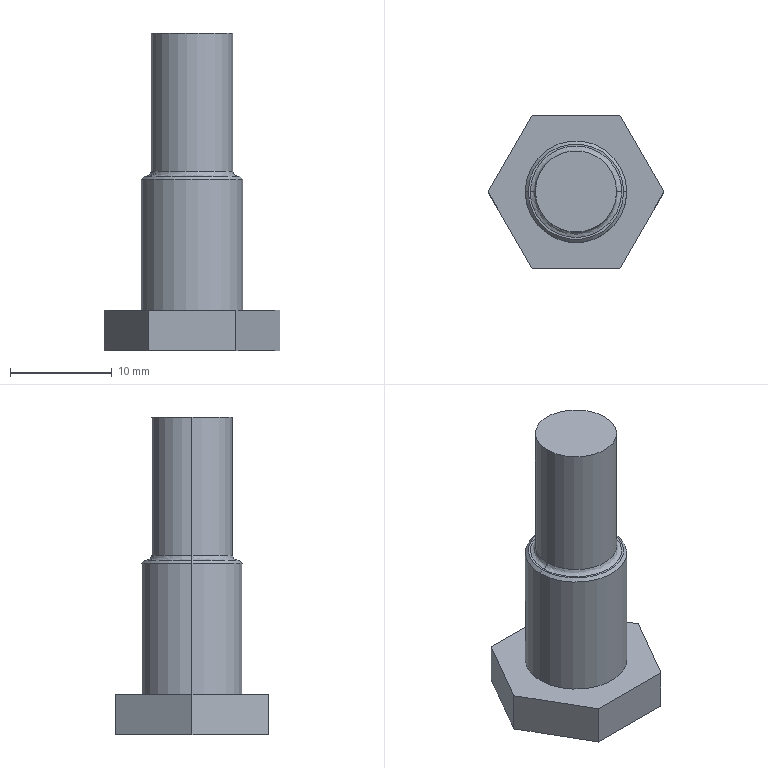Part | SolidWorks | features BaseBody 1 | 1 solid | 18 faces | box 17.321 x 15 x 31.3 mm | volume 2525 mm3 | plane 10 | cylinder 4 | spline 2 | cone 2 | commonest cylinder face diameters 8 x2 10 x2
STEP:
#1=CARTESIAN_POINT('',(-4.5,0.,17.2));
#2=VERTEX_POINT('',#1);
#3=CARTESIAN_POINT('',(4.5,0.,17.2));
#4=VERTEX_POINT('',#3);
#5=CARTESIAN_POINT('',(-4.5,0.,17.2));
#6=CARTESIAN_POINT('',(-4.5,0.286,17.2));
#7=CARTESIAN_POINT('',(-4.461,0.7076,17.2));
#8=CARTESIAN_POINT('',(-4.345,1.186,17.2));
#9=CARTESIAN_POINT('',(-4.27,1.422,17.2));
#10=CARTESIAN_POINT('',(-4.235,1.523,17.2));
#11=CARTESIAN_POINT('',(-4.21,1.59,17.2));
#12=CARTESIAN_POINT('',(-4.198,1.621,17.2));
#13=CARTESIAN_POINT('',(-4.128,1.798,17.2));
#14=CARTESIAN_POINT('',(-4.034,2.004,17.2));
#15=CARTESIAN_POINT('',(-3.925,2.203,17.2));
#16=CARTESIAN_POINT('',(-3.848,2.334,17.2));
#17=CARTESIAN_POINT('',(-3.809,2.398,17.2));
#18=CARTESIAN_POINT('',(-3.597,2.722,17.2));
#19=CARTESIAN_POINT('',(-3.401,2.963,17.2));
#20=CARTESIAN_POINT('',(-3.072,3.292,17.2));
#21=CARTESIAN_POINT('',(-2.9,3.447,17.2));
#22=CARTESIAN_POINT('',(-2.716,3.589,17.2));
#23=CARTESIAN_POINT('',(-2.591,3.68,17.2));
#24=CARTESIAN_POINT('',(-2.526,3.725,17.2));
#25=CARTESIAN_POINT('',(-2.335,3.85,17.2));
#26=CARTESIAN_POINT('',(-2.139,3.964,17.2));
#27=CARTESIAN_POINT('',(-1.901,4.08,17.2));
#28=CARTESIAN_POINT('',(-1.779,4.134,17.2));
#29=CARTESIAN_POINT('',(-1.727,4.155,17.2));
#30=CARTESIAN_POINT('',(-1.692,4.17,17.2));
#31=CARTESIAN_POINT('',(-1.673,4.177,17.2));
#32=CARTESIAN_POINT('',(-1.125,4.395,17.2));
#33=CARTESIAN_POINT('',(-0.5719,4.5,17.2));
#34=CARTESIAN_POINT('',(0.2859,4.5,17.2));
#35=CARTESIAN_POINT('',(0.7075,4.461,17.2));
#36=CARTESIAN_POINT('',(1.186,4.345,17.2));
#37=CARTESIAN_POINT('',(1.422,4.27,17.2));
#38=CARTESIAN_POINT('',(1.523,4.235,17.2));
#39=CARTESIAN_POINT('',(1.59,4.21,17.2));
#40=CARTESIAN_POINT('',(1.621,4.198,17.2));
#41=CARTESIAN_POINT('',(1.798,4.128,17.2));
#42=CARTESIAN_POINT('',(2.004,4.034,17.2));
#43=CARTESIAN_POINT('',(2.203,3.925,17.2));
#44=CARTESIAN_POINT('',(2.334,3.848,17.2));
#45=CARTESIAN_POINT('',(2.398,3.809,17.2));
#46=CARTESIAN_POINT('',(2.722,3.597,17.2));
#47=CARTESIAN_POINT('',(2.963,3.401,17.2));
#48=CARTESIAN_POINT('',(3.292,3.072,17.2));
#49=CARTESIAN_POINT('',(3.447,2.9,17.2));
#50=CARTESIAN_POINT('',(3.589,2.716,17.2));
#51=CARTESIAN_POINT('',(3.68,2.591,17.2));
#52=CARTESIAN_POINT('',(3.725,2.526,17.2));
#53=CARTESIAN_POINT('',(3.85,2.335,17.2));
#54=CARTESIAN_POINT('',(3.964,2.139,17.2));
#55=CARTESIAN_POINT('',(4.08,1.901,17.2));
#56=CARTESIAN_POINT('',(4.134,1.779,17.2));
#57=CARTESIAN_POINT('',(4.155,1.727,17.2));
#58=CARTESIAN_POINT('',(4.17,1.692,17.2));
#59=CARTESIAN_POINT('',(4.177,1.673,17.2));
#60=CARTESIAN_POINT('',(4.395,1.125,17.2));
#61=CARTESIAN_POINT('',(4.5,0.5724,17.2));
#62=CARTESIAN_POINT('',(4.5,0.,17.2));
#63=B_SPLINE_CURVE_WITH_KNOTS('',3,(#5,#6,#7,#8,#9,#10,#11,#12,#13,#14,#15,#16,#17,#18,#19,#20,#21,#22,#23,#24,#25,#26,#27,#28,#29,#30,#31,#32,#33,#34,#35,#36,#37,#38,#39,#40,#41,#42,#43,#44,#45,#46,#47,#48,#49,#50,#51,#52,#53,#54,#55,#56,#57,#58,#59,#60,#61,#62),.UNSPECIFIED.,.F.,.F.,(4,1,1,1,2,2,1,2,2,2,1,2,2,1,1,1,2,2,2,1,1,1,2,2,1,2,2,2,1,2,2,1,1,1,2,2,4),(0.,0.0625,0.09375,0.1094,0.1172,0.125,0.1562,0.1719,0.1875,0.25,0.2812,0.2969,0.3125,0.3437,0.3594,0.3672,0.3711,0.375,0.5,0.5625,0.5937,0.6094,0.6172,0.625,0.6562,0.6719,0.6875,0.75,0.7812,0.7969,0.8125,0.8437,0.8594,0.8672,0.8711,0.875,1.),.UNSPECIFIED.);
#64=EDGE_CURVE('',#2,#4,#63,.T.);
#65=ORIENTED_EDGE('',*,*,#64,.F.);
#66=CARTESIAN_POINT('',(-4.,0.,17.7));
#67=VERTEX_POINT('',#66);
#68=CARTESIAN_POINT('',(-4.5,0.,17.7));
#69=DIRECTION('',(0.,-1.,0.));
#70=DIRECTION('',(-1.,0.,0.));
#71=AXIS2_PLACEMENT_3D('',#68,#69,#70);
#72=CIRCLE('',#71,0.5);
#73=EDGE_CURVE('',#2,#67,#72,.T.);
#74=ORIENTED_EDGE('',*,*,#73,.T.);
#75=CARTESIAN_POINT('',(4.,0.,17.7));
#76=VERTEX_POINT('',#75);
#77=CARTESIAN_POINT('',(0.,0.,17.7));
#78=DIRECTION('',(0.,0.,1.));
#79=DIRECTION('',(1.,0.,0.));
#80=AXIS2_PLACEMENT_3D('',#77,#78,#79);
#81=CIRCLE('',#80,4.);
#82=EDGE_CURVE('',#76,#67,#81,.T.);
#83=ORIENTED_EDGE('',*,*,#82,.F.);
#84=CARTESIAN_POINT('',(4.5,0.,17.7));
#85=DIRECTION('',(0.,1.,0.));
#86=DIRECTION('',(1.,0.,0.));
#87=AXIS2_PLACEMENT_3D('',#84,#85,#86);
#88=CIRCLE('',#87,0.5);
#89=EDGE_CURVE('',#4,#76,#88,.T.);
#90=ORIENTED_EDGE('',*,*,#89,.F.);
#91=EDGE_LOOP('',(#65,#74,#83,#90));
#92=FACE_OUTER_BOUND('',#91,.T.);
#93=CARTESIAN_POINT('',(4.5,0.,17.2));
#94=CARTESIAN_POINT('',(4.5,9.,17.2));
#95=CARTESIAN_POINT('',(-4.5,9.,17.2));
#96=CARTESIAN_POINT('',(-4.5,0.,17.2));
#97=CARTESIAN_POINT('',(4.207,0.,17.2));
#98=CARTESIAN_POINT('',(4.207,8.414,17.2));
#99=CARTESIAN_POINT('',(-4.207,8.414,17.2));
#100=CARTESIAN_POINT('',(-4.207,0.,17.2));
#101=CARTESIAN_POINT('',(4.,0.,17.407));
#102=CARTESIAN_POINT('',(4.,8.,17.407));
#103=CARTESIAN_POINT('',(-4.,8.,17.407));
#104=CARTESIAN_POINT('',(-4.,0.,17.407));
#105=CARTESIAN_POINT('',(4.,0.,17.7));
#106=CARTESIAN_POINT('',(4.,8.,17.7));
#107=CARTESIAN_POINT('',(-4.,8.,17.7));
#108=CARTESIAN_POINT('',(-4.,0.,17.7));
#109=(BOUNDED_SURFACE()B_SPLINE_SURFACE(3,3,((#93,#94,#95,#96),(#97,#98,#99,#100),(#101,#102,#103,#104),(#105,#106,#107,#108)),.UNSPECIFIED.,.F.,.F.,.T.)B_SPLINE_SURFACE_WITH_KNOTS((4,4),(4,4),(0.,1.),(0.,1.),.UNSPECIFIED.)GEOMETRIC_REPRESENTATION_ITEM()RATIONAL_B_SPLINE_SURFACE(((1.,0.3333,0.3333,1.),(0.8047,0.2682,0.2682,0.8047),(0.8047,0.2682,0.2682,0.8047),(1.,0.3333,0.3333,1.)))REPRESENTATION_ITEM('')SURFACE());
#110=ADVANCED_FACE('',(#92),#109,.F.);
#111=CARTESIAN_POINT('',(-5.,0.,16.9));
#112=VERTEX_POINT('',#111);
#113=CARTESIAN_POINT('',(5.,0.,16.9));
#114=VERTEX_POINT('',#113);
#115=CARTESIAN_POINT('',(0.,0.,16.9));
#116=DIRECTION('',(0.,0.,-1.));
#117=DIRECTION('',(-1.,0.,0.));
#118=AXIS2_PLACEMENT_3D('',#115,#116,#117);
#119=CIRCLE('',#118,5.);
#120=EDGE_CURVE('',#112,#114,#119,.T.);
#121=ORIENTED_EDGE('',*,*,#120,.T.);
#122=CARTESIAN_POINT('',(5.,0.,4.));
#123=VERTEX_POINT('',#122);
#124=CARTESIAN_POINT('',(5.,0.,17.));
#125=DIRECTION('',(0.,0.,-1.));
#126=VECTOR('',#125,1000.);
#127=LINE('',#124,#126);
#128=EDGE_CURVE('',#114,#123,#127,.T.);
#129=ORIENTED_EDGE('',*,*,#128,.T.);
#130=CARTESIAN_POINT('',(-5.,0.,4.));
#131=VERTEX_POINT('',#130);
#132=CARTESIAN_POINT('',(0.,0.,4.));
#133=DIRECTION('',(0.,0.,1.));
#134=DIRECTION('',(-1.,0.,0.));
#135=AXIS2_PLACEMENT_3D('',#132,#133,#134);
#136=CIRCLE('',#135,5.);
#137=EDGE_CURVE('',#123,#131,#136,.T.);
#138=ORIENTED_EDGE('',*,*,#137,.T.);
#139=CARTESIAN_POINT('',(-5.,0.,17.));
#140=DIRECTION('',(0.,0.,-1.));
#141=VECTOR('',#140,1000.);
#142=LINE('',#139,#141);
#143=EDGE_CURVE('',#112,#131,#142,.T.);
#144=ORIENTED_EDGE('',*,*,#143,.F.);
#145=EDGE_LOOP('',(#121,#129,#138,#144));
#146=FACE_OUTER_BOUND('',#145,.T.);
#147=CARTESIAN_POINT('',(0.,0.,17.));
#148=DIRECTION('',(0.,0.,-1.));
#149=DIRECTION('',(-1.,0.,0.));
#150=AXIS2_PLACEMENT_3D('',#147,#148,#149);
#151=CYLINDRICAL_SURFACE('',#150,5.);
#152=ADVANCED_FACE('',(#146),#151,.T.);
#153=CARTESIAN_POINT('',(-4.7,0.,17.2));
#154=VERTEX_POINT('',#153);
#155=CARTESIAN_POINT('',(4.7,0.,17.2));
#156=VERTEX_POINT('',#155);
#157=CARTESIAN_POINT('',(0.,0.,17.2));
#158=DIRECTION('',(0.,0.,-1.));
#159=DIRECTION('',(-1.,0.,0.));
#160=AXIS2_PLACEMENT_3D('',#157,#158,#159);
#161=CIRCLE('',#160,4.7);
#162=EDGE_CURVE('',#154,#156,#161,.T.);
#163=ORIENTED_EDGE('',*,*,#162,.T.);
#164=CARTESIAN_POINT('',(5.,0.,16.9));
#165=DIRECTION('',(0.7071,0.,-0.7071));
#166=VECTOR('',#165,1000.);
#167=LINE('',#164,#166);
#168=EDGE_CURVE('',#156,#114,#167,.T.);
#169=ORIENTED_EDGE('',*,*,#168,.T.);
#170=ORIENTED_EDGE('',*,*,#120,.F.);
#171=CARTESIAN_POINT('',(-5.,0.,16.9));
#172=DIRECTION('',(-0.7071,0.,-0.7071));
#173=VECTOR('',#172,1000.);
#174=LINE('',#171,#173);
#175=EDGE_CURVE('',#154,#112,#174,.T.);
#176=ORIENTED_EDGE('',*,*,#175,.F.);
#177=EDGE_LOOP('',(#163,#169,#170,#176));
#178=FACE_OUTER_BOUND('',#177,.T.);
#179=CARTESIAN_POINT('',(0.,0.,16.9));
#180=DIRECTION('',(0.,0.,-1.));
#181=DIRECTION('',(-1.,0.,0.));
#182=AXIS2_PLACEMENT_3D('',#179,#180,#181);
#183=CONICAL_SURFACE('',#182,5.,0.7854);
#184=ADVANCED_FACE('',(#178),#183,.T.);
#185=CARTESIAN_POINT('',(-4.,0.,31.3));
#186=VERTEX_POINT('',#185);
#187=CARTESIAN_POINT('',(4.,0.,31.3));
#188=VERTEX_POINT('',#187);
#189=CARTESIAN_POINT('',(0.,0.,31.3));
#190=DIRECTION('',(0.,0.,-1.));
#191=DIRECTION('',(-1.,0.,0.));
#192=AXIS2_PLACEMENT_3D('',#189,#190,#191);
#193=CIRCLE('',#192,4.);
#194=EDGE_CURVE('',#186,#188,#193,.T.);
#195=ORIENTED_EDGE('',*,*,#194,.T.);
#196=CARTESIAN_POINT('',(4.,0.,31.3));
#197=DIRECTION('',(0.,0.,-1.));
#198=VECTOR('',#197,1000.);
#199=LINE('',#196,#198);
#200=EDGE_CURVE('',#188,#76,#199,.T.);
#201=ORIENTED_EDGE('',*,*,#200,.T.);
#202=ORIENTED_EDGE('',*,*,#82,.T.);
#203=CARTESIAN_POINT('',(-4.,0.,31.3));
#204=DIRECTION('',(0.,0.,-1.));
#205=VECTOR('',#204,1000.);
#206=LINE('',#203,#205);
#207=EDGE_CURVE('',#186,#67,#206,.T.);
#208=ORIENTED_EDGE('',*,*,#207,.F.);
#209=EDGE_LOOP('',(#195,#201,#202,#208));
#210=FACE_OUTER_BOUND('',#209,.T.);
#211=CARTESIAN_POINT('',(0.,0.,31.3));
#212=DIRECTION('',(0.,0.,-1.));
#213=DIRECTION('',(-1.,0.,0.));
#214=AXIS2_PLACEMENT_3D('',#211,#212,#213);
#215=CYLINDRICAL_SURFACE('',#214,4.);
#216=ADVANCED_FACE('',(#210),#215,.T.);
#217=ORIENTED_EDGE('',*,*,#128,.F.);
#218=CARTESIAN_POINT('',(0.,0.,16.9));
#219=DIRECTION('',(0.,0.,-1.));
#220=DIRECTION('',(-1.,0.,0.));
#221=AXIS2_PLACEMENT_3D('',#218,#219,#220);
#222=CIRCLE('',#221,5.);
#223=EDGE_CURVE('',#114,#112,#222,.T.);
#224=ORIENTED_EDGE('',*,*,#223,.T.);
#225=ORIENTED_EDGE('',*,*,#143,.T.);
#226=CARTESIAN_POINT('',(0.,0.,4.));
#227=DIRECTION('',(0.,0.,1.));
#228=DIRECTION('',(-1.,0.,0.));
#229=AXIS2_PLACEMENT_3D('',#226,#227,#228);
#230=CIRCLE('',#229,5.);
#231=EDGE_CURVE('',#131,#123,#230,.T.);
#232=ORIENTED_EDGE('',*,*,#231,.T.);
#233=EDGE_LOOP('',(#217,#224,#225,#232));
#234=FACE_OUTER_BOUND('',#233,.T.);
#235=CARTESIAN_POINT('',(0.,0.,17.));
#236=DIRECTION('',(0.,0.,-1.));
#237=DIRECTION('',(-1.,0.,0.));
#238=AXIS2_PLACEMENT_3D('',#235,#236,#237);
#239=CYLINDRICAL_SURFACE('',#238,5.);
#240=ADVANCED_FACE('',(#234),#239,.T.);
#241=CARTESIAN_POINT('',(-4.33,-7.5,4.));
#242=VERTEX_POINT('',#241);
#243=CARTESIAN_POINT('',(4.33,-7.5,4.));
#244=VERTEX_POINT('',#243);
#245=CARTESIAN_POINT('',(0.,-7.5,4.));
#246=DIRECTION('',(1.,0.,0.));
#247=VECTOR('',#246,1000.);
#248=LINE('',#245,#247);
#249=EDGE_CURVE('',#242,#244,#248,.T.);
#250=ORIENTED_EDGE('',*,*,#249,.T.);
#251=CARTESIAN_POINT('',(8.66,0.,4.));
#252=VERTEX_POINT('',#251);
#253=CARTESIAN_POINT('',(4.33,-7.5,4.));
#254=DIRECTION('',(0.5,0.866,0.));
#255=VECTOR('',#254,1000.);
#256=LINE('',#253,#255);
#257=EDGE_CURVE('',#244,#252,#256,.T.);
#258=ORIENTED_EDGE('',*,*,#257,.T.);
#259=CARTESIAN_POINT('',(4.33,7.5,4.));
#260=VERTEX_POINT('',#259);
#261=CARTESIAN_POINT('',(8.66,0.,4.));
#262=DIRECTION('',(-0.5,0.866,0.));
#263=VECTOR('',#262,1000.);
#264=LINE('',#261,#263);
#265=EDGE_CURVE('',#252,#260,#264,.T.);
#266=ORIENTED_EDGE('',*,*,#265,.T.);
#267=CARTESIAN_POINT('',(-4.33,7.5,4.));
#268=VERTEX_POINT('',#267);
#269=CARTESIAN_POINT('',(0.,7.5,4.));
#270=DIRECTION('',(-1.,0.,0.));
#271=VECTOR('',#270,1000.);
#272=LINE('',#269,#271);
#273=EDGE_CURVE('',#260,#268,#272,.T.);
#274=ORIENTED_EDGE('',*,*,#273,.T.);
#275=CARTESIAN_POINT('',(-8.66,0.,4.));
#276=VERTEX_POINT('',#275);
#277=CARTESIAN_POINT('',(-4.33,7.5,4.));
#278=DIRECTION('',(-0.5,-0.866,0.));
#279=VECTOR('',#278,1000.);
#280=LINE('',#277,#279);
#281=EDGE_CURVE('',#268,#276,#280,.T.);
#282=ORIENTED_EDGE('',*,*,#281,.T.);
#283=CARTESIAN_POINT('',(-8.66,0.,4.));
#284=DIRECTION('',(0.5,-0.866,0.));
#285=VECTOR('',#284,1000.);
#286=LINE('',#283,#285);
#287=EDGE_CURVE('',#276,#242,#286,.T.);
#288=ORIENTED_EDGE('',*,*,#287,.T.);
#289=EDGE_LOOP('',(#250,#258,#266,#274,#282,#288));
#290=FACE_OUTER_BOUND('',#289,.T.);
#291=ORIENTED_EDGE('',*,*,#231,.F.);
#292=ORIENTED_EDGE('',*,*,#137,.F.);
#293=EDGE_LOOP('',(#291,#292));
#294=FACE_BOUND('',#293,.T.);
#295=CARTESIAN_POINT('',(0.,0.,4.));
#296=DIRECTION('',(0.,0.,1.));
#297=DIRECTION('',(1.,0.,0.));
#298=AXIS2_PLACEMENT_3D('',#295,#296,#297);
#299=PLANE('',#298);
#300=ADVANCED_FACE('',(#290,#294),#299,.T.);
#301=ORIENTED_EDGE('',*,*,#168,.F.);
#302=CARTESIAN_POINT('',(0.,0.,17.2));
#303=DIRECTION('',(0.,0.,-1.));
#304=DIRECTION('',(-1.,0.,0.));
#305=AXIS2_PLACEMENT_3D('',#302,#303,#304);
#306=CIRCLE('',#305,4.7);
#307=EDGE_CURVE('',#156,#154,#306,.T.);
#308=ORIENTED_EDGE('',*,*,#307,.T.);
#309=ORIENTED_EDGE('',*,*,#175,.T.);
#310=ORIENTED_EDGE('',*,*,#223,.F.);
#311=EDGE_LOOP('',(#301,#308,#309,#310));
#312=FACE_OUTER_BOUND('',#311,.T.);
#313=CARTESIAN_POINT('',(0.,0.,16.9));
#314=DIRECTION('',(0.,0.,-1.));
#315=DIRECTION('',(-1.,0.,0.));
#316=AXIS2_PLACEMENT_3D('',#313,#314,#315);
#317=CONICAL_SURFACE('',#316,5.,0.7854);
#318=ADVANCED_FACE('',(#312),#317,.T.);
#319=CARTESIAN_POINT('',(8.66,0.,0.));
#320=VERTEX_POINT('',#319);
#321=CARTESIAN_POINT('',(8.66,0.,4.));
#322=DIRECTION('',(0.,0.,-1.));
#323=VECTOR('',#322,1000.);
#324=LINE('',#321,#323);
#325=EDGE_CURVE('',#252,#320,#324,.T.);
#326=ORIENTED_EDGE('',*,*,#325,.F.);
#327=ORIENTED_EDGE('',*,*,#257,.F.);
#328=CARTESIAN_POINT('',(4.33,-7.5,0.));
#329=VERTEX_POINT('',#328);
#330=CARTESIAN_POINT('',(4.33,-7.5,4.));
#331=DIRECTION('',(0.,0.,1.));
#332=VECTOR('',#331,1000.);
#333=LINE('',#330,#332);
#334=EDGE_CURVE('',#329,#244,#333,.T.);
#335=ORIENTED_EDGE('',*,*,#334,.F.);
#336=CARTESIAN_POINT('',(4.33,-7.5,0.));
#337=DIRECTION('',(-0.5,-0.866,0.));
#338=VECTOR('',#337,1000.);
#339=LINE('',#336,#338);
#340=EDGE_CURVE('',#320,#329,#339,.T.);
#341=ORIENTED_EDGE('',*,*,#340,.F.);
#342=EDGE_LOOP('',(#326,#327,#335,#341));
#343=FACE_OUTER_BOUND('',#342,.T.);
#344=CARTESIAN_POINT('',(4.33,-7.5,4.));
#345=DIRECTION('',(-0.866,0.5,0.));
#346=DIRECTION('',(-0.5,-0.866,0.));
#347=AXIS2_PLACEMENT_3D('',#344,#345,#346);
#348=PLANE('',#347);
#349=ADVANCED_FACE('',(#343),#348,.F.);
#350=ORIENTED_EDGE('',*,*,#334,.T.);
#351=ORIENTED_EDGE('',*,*,#249,.F.);
#352=CARTESIAN_POINT('',(-4.33,-7.5,0.));
#353=VERTEX_POINT('',#352);
#354=CARTESIAN_POINT('',(-4.33,-7.5,4.));
#355=DIRECTION('',(0.,0.,1.));
#356=VECTOR('',#355,1000.);
#357=LINE('',#354,#356);
#358=EDGE_CURVE('',#353,#242,#357,.T.);
#359=ORIENTED_EDGE('',*,*,#358,.F.);
#360=CARTESIAN_POINT('',(-4.33,-7.5,0.));
#361=DIRECTION('',(-1.,0.,0.));
#362=VECTOR('',#361,1000.);
#363=LINE('',#360,#362);
#364=EDGE_CURVE('',#329,#353,#363,.T.);
#365=ORIENTED_EDGE('',*,*,#364,.F.);
#366=EDGE_LOOP('',(#350,#351,#359,#365));
#367=FACE_OUTER_BOUND('',#366,.T.);
#368=CARTESIAN_POINT('',(-4.33,-7.5,4.));
#369=DIRECTION('',(0.,1.,0.));
#370=DIRECTION('',(-1.,0.,0.));
#371=AXIS2_PLACEMENT_3D('',#368,#369,#370);
#372=PLANE('',#371);
#373=ADVANCED_FACE('',(#367),#372,.F.);
#374=ORIENTED_EDGE('',*,*,#358,.T.);
#375=ORIENTED_EDGE('',*,*,#287,.F.);
#376=CARTESIAN_POINT('',(-8.66,0.,0.));
#377=VERTEX_POINT('',#376);
#378=CARTESIAN_POINT('',(-8.66,0.,4.));
#379=DIRECTION('',(0.,0.,1.));
#380=VECTOR('',#379,1000.);
#381=LINE('',#378,#380);
#382=EDGE_CURVE('',#377,#276,#381,.T.);
#383=ORIENTED_EDGE('',*,*,#382,.F.);
#384=CARTESIAN_POINT('',(-8.66,0.,0.));
#385=DIRECTION('',(-0.5,0.866,0.));
#386=VECTOR('',#385,1000.);
#387=LINE('',#384,#386);
#388=EDGE_CURVE('',#353,#377,#387,.T.);
#389=ORIENTED_EDGE('',*,*,#388,.F.);
#390=EDGE_LOOP('',(#374,#375,#383,#389));
#391=FACE_OUTER_BOUND('',#390,.T.);
#392=CARTESIAN_POINT('',(-8.66,0.,4.));
#393=DIRECTION('',(0.866,0.5,0.));
#394=DIRECTION('',(-0.5,0.866,0.));
#395=AXIS2_PLACEMENT_3D('',#392,#393,#394);
#396=PLANE('',#395);
#397=ADVANCED_FACE('',(#391),#396,.F.);
#398=ORIENTED_EDGE('',*,*,#382,.T.);
#399=ORIENTED_EDGE('',*,*,#281,.F.);
#400=CARTESIAN_POINT('',(-4.33,7.5,0.));
#401=VERTEX_POINT('',#400);
#402=CARTESIAN_POINT('',(-4.33,7.5,4.));
#403=DIRECTION('',(0.,0.,1.));
#404=VECTOR('',#403,1000.);
#405=LINE('',#402,#404);
#406=EDGE_CURVE('',#401,#268,#405,.T.);
#407=ORIENTED_EDGE('',*,*,#406,.F.);
#408=CARTESIAN_POINT('',(-4.33,7.5,0.));
#409=DIRECTION('',(0.5,0.866,0.));
#410=VECTOR('',#409,1000.);
#411=LINE('',#408,#410);
#412=EDGE_CURVE('',#377,#401,#411,.T.);
#413=ORIENTED_EDGE('',*,*,#412,.F.);
#414=EDGE_LOOP('',(#398,#399,#407,#413));
#415=FACE_OUTER_BOUND('',#414,.T.);
#416=CARTESIAN_POINT('',(-4.33,7.5,4.));
#417=DIRECTION('',(0.866,-0.5,0.));
#418=DIRECTION('',(0.5,0.866,0.));
#419=AXIS2_PLACEMENT_3D('',#416,#417,#418);
#420=PLANE('',#419);
#421=ADVANCED_FACE('',(#415),#420,.F.);
#422=ORIENTED_EDGE('',*,*,#406,.T.);
#423=ORIENTED_EDGE('',*,*,#273,.F.);
#424=CARTESIAN_POINT('',(4.33,7.5,0.));
#425=VERTEX_POINT('',#424);
#426=CARTESIAN_POINT('',(4.33,7.5,4.));
#427=DIRECTION('',(0.,0.,1.));
#428=VECTOR('',#427,1000.);
#429=LINE('',#426,#428);
#430=EDGE_CURVE('',#425,#260,#429,.T.);
#431=ORIENTED_EDGE('',*,*,#430,.F.);
#432=CARTESIAN_POINT('',(4.33,7.5,0.));
#433=DIRECTION('',(1.,0.,0.));
#434=VECTOR('',#433,1000.);
#435=LINE('',#432,#434);
#436=EDGE_CURVE('',#401,#425,#435,.T.);
#437=ORIENTED_EDGE('',*,*,#436,.F.);
#438=EDGE_LOOP('',(#422,#423,#431,#437));
#439=FACE_OUTER_BOUND('',#438,.T.);
#440=CARTESIAN_POINT('',(4.33,7.5,4.));
#441=DIRECTION('',(0.,-1.,0.));
#442=DIRECTION('',(0.,0.,-1.));
#443=AXIS2_PLACEMENT_3D('',#440,#441,#442);
#444=PLANE('',#443);
#445=ADVANCED_FACE('',(#439),#444,.F.);
#446=ORIENTED_EDGE('',*,*,#430,.T.);
#447=ORIENTED_EDGE('',*,*,#265,.F.);
#448=ORIENTED_EDGE('',*,*,#325,.T.);
#449=CARTESIAN_POINT('',(8.66,0.,0.));
#450=DIRECTION('',(0.5,-0.866,0.));
#451=VECTOR('',#450,1000.);
#452=LINE('',#449,#451);
#453=EDGE_CURVE('',#425,#320,#452,.T.);
#454=ORIENTED_EDGE('',*,*,#453,.F.);
#455=EDGE_LOOP('',(#446,#447,#448,#454));
#456=FACE_OUTER_BOUND('',#455,.T.);
#457=CARTESIAN_POINT('',(8.66,0.,4.));
#458=DIRECTION('',(-0.866,-0.5,0.));
#459=DIRECTION('',(0.5,-0.866,0.));
#460=AXIS2_PLACEMENT_3D('',#457,#458,#459);
#461=PLANE('',#460);
#462=ADVANCED_FACE('',(#456),#461,.F.);
#463=CARTESIAN_POINT('',(4.5,0.,17.2));
#464=CARTESIAN_POINT('',(4.5,-0.286,17.2));
#465=CARTESIAN_POINT('',(4.461,-0.7076,17.2));
#466=CARTESIAN_POINT('',(4.345,-1.186,17.2));
#467=CARTESIAN_POINT('',(4.27,-1.422,17.2));
#468=CARTESIAN_POINT('',(4.235,-1.523,17.2));
#469=CARTESIAN_POINT('',(4.21,-1.59,17.2));
#470=CARTESIAN_POINT('',(4.198,-1.621,17.2));
#471=CARTESIAN_POINT('',(4.128,-1.798,17.2));
#472=CARTESIAN_POINT('',(4.034,-2.004,17.2));
#473=CARTESIAN_POINT('',(3.925,-2.203,17.2));
#474=CARTESIAN_POINT('',(3.848,-2.334,17.2));
#475=CARTESIAN_POINT('',(3.809,-2.398,17.2));
#476=CARTESIAN_POINT('',(3.597,-2.722,17.2));
#477=CARTESIAN_POINT('',(3.401,-2.963,17.2));
#478=CARTESIAN_POINT('',(3.072,-3.292,17.2));
#479=CARTESIAN_POINT('',(2.9,-3.447,17.2));
#480=CARTESIAN_POINT('',(2.716,-3.589,17.2));
#481=CARTESIAN_POINT('',(2.591,-3.68,17.2));
#482=CARTESIAN_POINT('',(2.526,-3.725,17.2));
#483=CARTESIAN_POINT('',(2.335,-3.85,17.2));
#484=CARTESIAN_POINT('',(2.139,-3.964,17.2));
#485=CARTESIAN_POINT('',(1.901,-4.08,17.2));
#486=CARTESIAN_POINT('',(1.779,-4.134,17.2));
#487=CARTESIAN_POINT('',(1.727,-4.155,17.2));
#488=CARTESIAN_POINT('',(1.692,-4.17,17.2));
#489=CARTESIAN_POINT('',(1.673,-4.177,17.2));
#490=CARTESIAN_POINT('',(1.125,-4.395,17.2));
#491=CARTESIAN_POINT('',(0.5719,-4.5,17.2));
#492=CARTESIAN_POINT('',(-0.2859,-4.5,17.2));
#493=CARTESIAN_POINT('',(-0.7075,-4.461,17.2));
#494=CARTESIAN_POINT('',(-1.186,-4.345,17.2));
#495=CARTESIAN_POINT('',(-1.422,-4.27,17.2));
#496=CARTESIAN_POINT('',(-1.523,-4.235,17.2));
#497=CARTESIAN_POINT('',(-1.59,-4.21,17.2));
#498=CARTESIAN_POINT('',(-1.621,-4.198,17.2));
#499=CARTESIAN_POINT('',(-1.798,-4.128,17.2));
#500=CARTESIAN_POINT('',(-2.004,-4.034,17.2));
#501=CARTESIAN_POINT('',(-2.203,-3.925,17.2));
#502=CARTESIAN_POINT('',(-2.334,-3.848,17.2));
#503=CARTESIAN_POINT('',(-2.398,-3.809,17.2));
#504=CARTESIAN_POINT('',(-2.722,-3.597,17.2));
#505=CARTESIAN_POINT('',(-2.963,-3.401,17.2));
#506=CARTESIAN_POINT('',(-3.292,-3.072,17.2));
#507=CARTESIAN_POINT('',(-3.447,-2.9,17.2));
#508=CARTESIAN_POINT('',(-3.589,-2.716,17.2));
#509=CARTESIAN_POINT('',(-3.68,-2.591,17.2));
#510=CARTESIAN_POINT('',(-3.725,-2.526,17.2));
#511=CARTESIAN_POINT('',(-3.85,-2.335,17.2));
#512=CARTESIAN_POINT('',(-3.964,-2.139,17.2));
#513=CARTESIAN_POINT('',(-4.08,-1.901,17.2));
#514=CARTESIAN_POINT('',(-4.134,-1.779,17.2));
#515=CARTESIAN_POINT('',(-4.155,-1.727,17.2));
#516=CARTESIAN_POINT('',(-4.17,-1.692,17.2));
#517=CARTESIAN_POINT('',(-4.177,-1.673,17.2));
#518=CARTESIAN_POINT('',(-4.395,-1.125,17.2));
#519=CARTESIAN_POINT('',(-4.5,-0.5724,17.2));
#520=CARTESIAN_POINT('',(-4.5,0.,17.2));
#521=B_SPLINE_CURVE_WITH_KNOTS('',3,(#463,#464,#465,#466,#467,#468,#469,#470,#471,#472,#473,#474,#475,#476,#477,#478,#479,#480,#481,#482,#483,#484,#485,#486,#487,#488,#489,#490,#491,#492,#493,#494,#495,#496,#497,#498,#499,#500,#501,#502,#503,#504,#505,#506,#507,#508,#509,#510,#511,#512,#513,#514,#515,#516,#517,#518,#519,#520),.UNSPECIFIED.,.F.,.F.,(4,1,1,1,2,2,1,2,2,2,1,2,2,1,1,1,2,2,2,1,1,1,2,2,1,2,2,2,1,2,2,1,1,1,2,2,4),(0.,0.0625,0.09375,0.1094,0.1172,0.125,0.1562,0.1719,0.1875,0.25,0.2812,0.2969,0.3125,0.3437,0.3594,0.3672,0.3711,0.375,0.5,0.5625,0.5937,0.6094,0.6172,0.625,0.6562,0.6719,0.6875,0.75,0.7813,0.7969,0.8125,0.8438,0.8594,0.8672,0.8711,0.875,1.),.UNSPECIFIED.);
#522=EDGE_CURVE('',#4,#2,#521,.T.);
#523=ORIENTED_EDGE('',*,*,#522,.T.);
#524=ORIENTED_EDGE('',*,*,#64,.T.);
#525=EDGE_LOOP('',(#523,#524));
#526=FACE_BOUND('',#525,.T.);
#527=ORIENTED_EDGE('',*,*,#162,.F.);
#528=ORIENTED_EDGE('',*,*,#307,.F.);
#529=EDGE_LOOP('',(#527,#528));
#530=FACE_OUTER_BOUND('',#529,.T.);
#531=CARTESIAN_POINT('',(0.,0.,17.2));
#532=DIRECTION('',(0.,0.,1.));
#533=DIRECTION('',(1.,0.,0.));
#534=AXIS2_PLACEMENT_3D('',#531,#532,#533);
#535=PLANE('',#534);
#536=ADVANCED_FACE('',(#526,#530),#535,.T.);
#537=ORIENTED_EDGE('',*,*,#340,.T.);
#538=ORIENTED_EDGE('',*,*,#364,.T.);
#539=ORIENTED_EDGE('',*,*,#388,.T.);
#540=ORIENTED_EDGE('',*,*,#412,.T.);
#541=ORIENTED_EDGE('',*,*,#436,.T.);
#542=ORIENTED_EDGE('',*,*,#453,.T.);
#543=EDGE_LOOP('',(#537,#538,#539,#540,#541,#542));
#544=FACE_OUTER_BOUND('',#543,.T.);
#545=CARTESIAN_POINT('',(0.,0.,0.));
#546=DIRECTION('',(0.,0.,1.));
#547=DIRECTION('',(1.,0.,0.));
#548=AXIS2_PLACEMENT_3D('',#545,#546,#547);
#549=PLANE('',#548);
#550=ADVANCED_FACE('',(#544),#549,.F.);
#551=ORIENTED_EDGE('',*,*,#73,.F.);
#552=ORIENTED_EDGE('',*,*,#522,.F.);
#553=ORIENTED_EDGE('',*,*,#89,.T.);
#554=CARTESIAN_POINT('',(0.,0.,17.7));
#555=DIRECTION('',(0.,0.,1.));
#556=DIRECTION('',(1.,0.,0.));
#557=AXIS2_PLACEMENT_3D('',#554,#555,#556);
#558=CIRCLE('',#557,4.);
#559=EDGE_CURVE('',#67,#76,#558,.T.);
#560=ORIENTED_EDGE('',*,*,#559,.F.);
#561=EDGE_LOOP('',(#551,#552,#553,#560));
#562=FACE_OUTER_BOUND('',#561,.T.);
#563=CARTESIAN_POINT('',(-4.5,0.,17.2));
#564=CARTESIAN_POINT('',(-4.5,-9.,17.2));
#565=CARTESIAN_POINT('',(4.5,-9.,17.2));
#566=CARTESIAN_POINT('',(4.5,0.,17.2));
#567=CARTESIAN_POINT('',(-4.207,0.,17.2));
#568=CARTESIAN_POINT('',(-4.207,-8.414,17.2));
#569=CARTESIAN_POINT('',(4.207,-8.414,17.2));
#570=CARTESIAN_POINT('',(4.207,0.,17.2));
#571=CARTESIAN_POINT('',(-4.,0.,17.407));
#572=CARTESIAN_POINT('',(-4.,-8.,17.407));
#573=CARTESIAN_POINT('',(4.,-8.,17.407));
#574=CARTESIAN_POINT('',(4.,0.,17.407));
#575=CARTESIAN_POINT('',(-4.,0.,17.7));
#576=CARTESIAN_POINT('',(-4.,-8.,17.7));
#577=CARTESIAN_POINT('',(4.,-8.,17.7));
#578=CARTESIAN_POINT('',(4.,0.,17.7));
#579=(BOUNDED_SURFACE()B_SPLINE_SURFACE(3,3,((#563,#564,#565,#566),(#567,#568,#569,#570),(#571,#572,#573,#574),(#575,#576,#577,#578)),.UNSPECIFIED.,.F.,.F.,.F.)B_SPLINE_SURFACE_WITH_KNOTS((4,4),(4,4),(0.,1.),(0.,1.),.UNSPECIFIED.)GEOMETRIC_REPRESENTATION_ITEM()RATIONAL_B_SPLINE_SURFACE(((1.,0.3333,0.3333,1.),(0.8047,0.2682,0.2682,0.8047),(0.8047,0.2682,0.2682,0.8047),(1.,0.3333,0.3333,1.)))REPRESENTATION_ITEM('')SURFACE());
#580=ADVANCED_FACE('',(#562),#579,.F.);
#581=ORIENTED_EDGE('',*,*,#200,.F.);
#582=CARTESIAN_POINT('',(0.,0.,31.3));
#583=DIRECTION('',(0.,0.,-1.));
#584=DIRECTION('',(-1.,0.,0.));
#585=AXIS2_PLACEMENT_3D('',#582,#583,#584);
#586=CIRCLE('',#585,4.);
#587=EDGE_CURVE('',#188,#186,#586,.T.);
#588=ORIENTED_EDGE('',*,*,#587,.T.);
#589=ORIENTED_EDGE('',*,*,#207,.T.);
#590=ORIENTED_EDGE('',*,*,#559,.T.);
#591=EDGE_LOOP('',(#581,#588,#589,#590));
#592=FACE_OUTER_BOUND('',#591,.T.);
#593=CARTESIAN_POINT('',(0.,0.,31.3));
#594=DIRECTION('',(0.,0.,-1.));
#595=DIRECTION('',(-1.,0.,0.));
#596=AXIS2_PLACEMENT_3D('',#593,#594,#595);
#597=CYLINDRICAL_SURFACE('',#596,4.);
#598=ADVANCED_FACE('',(#592),#597,.T.);
#599=ORIENTED_EDGE('',*,*,#194,.F.);
#600=ORIENTED_EDGE('',*,*,#587,.F.);
#601=EDGE_LOOP('',(#599,#600));
#602=FACE_OUTER_BOUND('',#601,.T.);
#603=CARTESIAN_POINT('',(0.,0.,31.3));
#604=DIRECTION('',(0.,0.,1.));
#605=DIRECTION('',(1.,0.,0.));
#606=AXIS2_PLACEMENT_3D('',#603,#604,#605);
#607=PLANE('',#606);
#608=ADVANCED_FACE('',(#602),#607,.T.);
#609=CLOSED_SHELL('',(#110,#152,#184,#216,#240,#300,#318,#349,#373,#397,#421,#445,#462,#536,#550,#580,#598,#608));
#610=MANIFOLD_SOLID_BREP('',#609);
#611=CARTESIAN_POINT('',(0.,0.,0.));
#612=DIRECTION('',(0.,0.,1.));
#613=DIRECTION('',(1.,0.,0.));
#614=AXIS2_PLACEMENT_3D('',#611,#612,#613);
#615=(LENGTH_UNIT()NAMED_UNIT(*)SI_UNIT(.MILLI.,.METRE.));
#616=UNCERTAINTY_MEASURE_WITH_UNIT(LENGTH_MEASURE(0.00001),#615,'','');
#617=(NAMED_UNIT(*)PLANE_ANGLE_UNIT()SI_UNIT($,.RADIAN.));
#618=(NAMED_UNIT(*)SI_UNIT($,.STERADIAN.)SOLID_ANGLE_UNIT());
#619=(GEOMETRIC_REPRESENTATION_CONTEXT(3)GLOBAL_UNCERTAINTY_ASSIGNED_CONTEXT((#616))GLOBAL_UNIT_ASSIGNED_CONTEXT((#615,#617,#618))REPRESENTATION_CONTEXT('',''));
#620=ADVANCED_BREP_SHAPE_REPRESENTATION('',(#610,#614),#619);